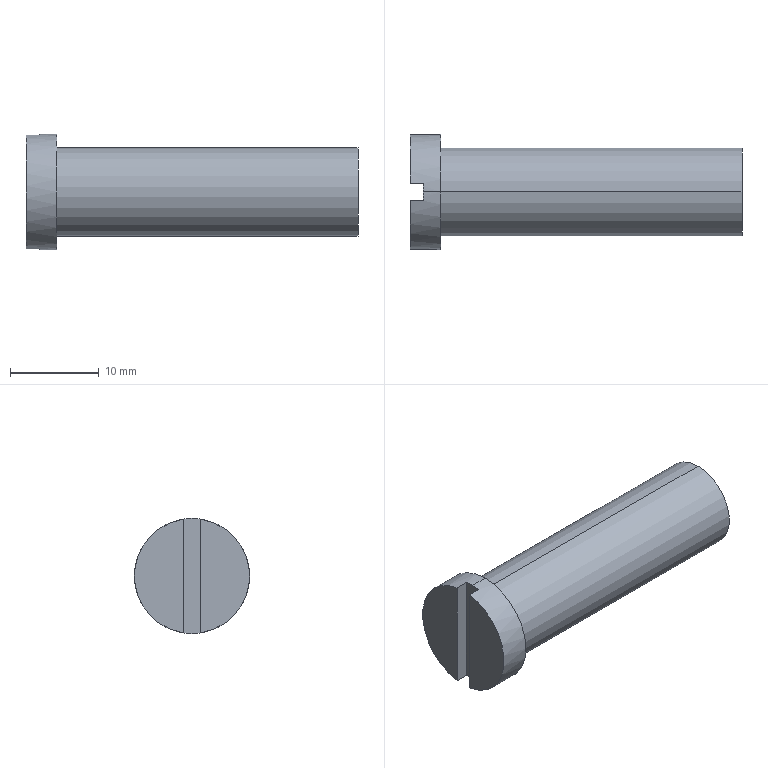Part | SolidWorks | features Chamfer 1, Cut 1, ICE 1, Revolution 1 | 1 solid | 11 faces | box 37.5 x 13 x 13 mm | volume 3096 mm3 | plane 7 | cylinder 4 | commonest cylinder face diameters 10 x2 13 x2
STEP:
#1=CARTESIAN_POINT('',(3.5,0.,6.5));
#2=VERTEX_POINT('',#1);
#3=CARTESIAN_POINT('',(3.5,0.,-6.5));
#4=VERTEX_POINT('',#3);
#5=CARTESIAN_POINT('',(3.5,0.,0.));
#6=DIRECTION('',(-1.,0.,0.));
#7=DIRECTION('',(0.,0.,1.));
#8=AXIS2_PLACEMENT_3D('',#5,#6,#7);
#9=CIRCLE('',#8,6.5);
#10=EDGE_CURVE('',#2,#4,#9,.T.);
#11=ORIENTED_EDGE('',*,*,#10,.T.);
#12=CARTESIAN_POINT('',(1.5,0.,-6.5));
#13=VERTEX_POINT('',#12);
#14=CARTESIAN_POINT('',(-19.421,0.,-6.5));
#15=DIRECTION('',(-1.,0.,0.));
#16=VECTOR('',#15,1000.);
#17=LINE('',#14,#16);
#18=EDGE_CURVE('',#4,#13,#17,.T.);
#19=ORIENTED_EDGE('',*,*,#18,.T.);
#20=CARTESIAN_POINT('',(1.5,1.,-6.423));
#21=VERTEX_POINT('',#20);
#22=CARTESIAN_POINT('',(1.5,0.,0.));
#23=DIRECTION('',(1.,0.,0.));
#24=DIRECTION('',(0.,1.,0.));
#25=AXIS2_PLACEMENT_3D('',#22,#23,#24);
#26=CIRCLE('',#25,6.5);
#27=EDGE_CURVE('',#13,#21,#26,.T.);
#28=ORIENTED_EDGE('',*,*,#27,.T.);
#29=CARTESIAN_POINT('',(0.,1.,-6.423));
#30=VERTEX_POINT('',#29);
#31=CARTESIAN_POINT('',(-19.421,1.,-6.423));
#32=DIRECTION('',(-1.,0.,0.));
#33=VECTOR('',#32,1000.);
#34=LINE('',#31,#33);
#35=EDGE_CURVE('',#21,#30,#34,.T.);
#36=ORIENTED_EDGE('',*,*,#35,.T.);
#37=CARTESIAN_POINT('',(0.,1.,6.423));
#38=VERTEX_POINT('',#37);
#39=CARTESIAN_POINT('',(0.,0.,0.));
#40=DIRECTION('',(-1.,0.,0.));
#41=DIRECTION('',(0.,0.,1.));
#42=AXIS2_PLACEMENT_3D('',#39,#40,#41);
#43=CIRCLE('',#42,6.5);
#44=EDGE_CURVE('',#38,#30,#43,.T.);
#45=ORIENTED_EDGE('',*,*,#44,.F.);
#46=CARTESIAN_POINT('',(1.5,1.,6.423));
#47=VERTEX_POINT('',#46);
#48=CARTESIAN_POINT('',(-19.421,1.,6.423));
#49=DIRECTION('',(1.,0.,0.));
#50=VECTOR('',#49,1000.);
#51=LINE('',#48,#50);
#52=EDGE_CURVE('',#38,#47,#51,.T.);
#53=ORIENTED_EDGE('',*,*,#52,.T.);
#54=CARTESIAN_POINT('',(1.5,0.,6.5));
#55=VERTEX_POINT('',#54);
#56=CARTESIAN_POINT('',(1.5,0.,0.));
#57=DIRECTION('',(1.,0.,0.));
#58=DIRECTION('',(0.,1.,0.));
#59=AXIS2_PLACEMENT_3D('',#56,#57,#58);
#60=CIRCLE('',#59,6.5);
#61=EDGE_CURVE('',#47,#55,#60,.T.);
#62=ORIENTED_EDGE('',*,*,#61,.T.);
#63=CARTESIAN_POINT('',(-19.421,0.,6.5));
#64=DIRECTION('',(-1.,0.,0.));
#65=VECTOR('',#64,1000.);
#66=LINE('',#63,#65);
#67=EDGE_CURVE('',#2,#55,#66,.T.);
#68=ORIENTED_EDGE('',*,*,#67,.F.);
#69=EDGE_LOOP('',(#11,#19,#28,#36,#45,#53,#62,#68));
#70=FACE_OUTER_BOUND('',#69,.T.);
#71=CARTESIAN_POINT('',(-19.421,0.,0.));
#72=DIRECTION('',(-1.,0.,0.));
#73=DIRECTION('',(0.,0.,1.));
#74=AXIS2_PLACEMENT_3D('',#71,#72,#73);
#75=CYLINDRICAL_SURFACE('',#74,6.5);
#76=ADVANCED_FACE('',(#70),#75,.T.);
#77=CARTESIAN_POINT('',(37.5,0.,-5.));
#78=VERTEX_POINT('',#77);
#79=CARTESIAN_POINT('',(37.5,0.,5.));
#80=VERTEX_POINT('',#79);
#81=CARTESIAN_POINT('',(37.5,0.,0.));
#82=DIRECTION('',(1.,0.,0.));
#83=DIRECTION('',(0.,0.,-1.));
#84=AXIS2_PLACEMENT_3D('',#81,#82,#83);
#85=CIRCLE('',#84,5.);
#86=EDGE_CURVE('',#78,#80,#85,.T.);
#87=ORIENTED_EDGE('',*,*,#86,.F.);
#88=CARTESIAN_POINT('',(3.5,0.,-5.));
#89=VERTEX_POINT('',#88);
#90=CARTESIAN_POINT('',(-19.421,0.,-5.));
#91=DIRECTION('',(-1.,0.,0.));
#92=VECTOR('',#91,1000.);
#93=LINE('',#90,#92);
#94=EDGE_CURVE('',#78,#89,#93,.T.);
#95=ORIENTED_EDGE('',*,*,#94,.T.);
#96=CARTESIAN_POINT('',(3.5,0.,5.));
#97=VERTEX_POINT('',#96);
#98=CARTESIAN_POINT('',(3.5,0.,0.));
#99=DIRECTION('',(-1.,0.,0.));
#100=DIRECTION('',(0.,0.,1.));
#101=AXIS2_PLACEMENT_3D('',#98,#99,#100);
#102=CIRCLE('',#101,5.);
#103=EDGE_CURVE('',#97,#89,#102,.T.);
#104=ORIENTED_EDGE('',*,*,#103,.F.);
#105=CARTESIAN_POINT('',(-19.421,0.,5.));
#106=DIRECTION('',(-1.,0.,0.));
#107=VECTOR('',#106,1000.);
#108=LINE('',#105,#107);
#109=EDGE_CURVE('',#80,#97,#108,.T.);
#110=ORIENTED_EDGE('',*,*,#109,.F.);
#111=EDGE_LOOP('',(#87,#95,#104,#110));
#112=FACE_OUTER_BOUND('',#111,.T.);
#113=CARTESIAN_POINT('',(-19.421,0.,0.));
#114=DIRECTION('',(-1.,0.,0.));
#115=DIRECTION('',(0.,0.,1.));
#116=AXIS2_PLACEMENT_3D('',#113,#114,#115);
#117=CYLINDRICAL_SURFACE('',#116,5.);
#118=ADVANCED_FACE('',(#112),#117,.T.);
#119=ORIENTED_EDGE('',*,*,#94,.F.);
#120=CARTESIAN_POINT('',(37.5,0.,0.));
#121=DIRECTION('',(1.,0.,0.));
#122=DIRECTION('',(0.,0.,-1.));
#123=AXIS2_PLACEMENT_3D('',#120,#121,#122);
#124=CIRCLE('',#123,5.);
#125=EDGE_CURVE('',#80,#78,#124,.T.);
#126=ORIENTED_EDGE('',*,*,#125,.F.);
#127=ORIENTED_EDGE('',*,*,#109,.T.);
#128=CARTESIAN_POINT('',(3.5,0.,0.));
#129=DIRECTION('',(-1.,0.,0.));
#130=DIRECTION('',(0.,0.,1.));
#131=AXIS2_PLACEMENT_3D('',#128,#129,#130);
#132=CIRCLE('',#131,5.);
#133=EDGE_CURVE('',#89,#97,#132,.T.);
#134=ORIENTED_EDGE('',*,*,#133,.F.);
#135=EDGE_LOOP('',(#119,#126,#127,#134));
#136=FACE_OUTER_BOUND('',#135,.T.);
#137=CARTESIAN_POINT('',(-19.421,0.,0.));
#138=DIRECTION('',(-1.,0.,0.));
#139=DIRECTION('',(0.,0.,1.));
#140=AXIS2_PLACEMENT_3D('',#137,#138,#139);
#141=CYLINDRICAL_SURFACE('',#140,5.);
#142=ADVANCED_FACE('',(#136),#141,.T.);
#143=CARTESIAN_POINT('',(0.,-1.,-6.423));
#144=VERTEX_POINT('',#143);
#145=CARTESIAN_POINT('',(0.,-1.,6.423));
#146=VERTEX_POINT('',#145);
#147=CARTESIAN_POINT('',(0.,0.,0.));
#148=DIRECTION('',(-1.,0.,0.));
#149=DIRECTION('',(0.,0.,1.));
#150=AXIS2_PLACEMENT_3D('',#147,#148,#149);
#151=CIRCLE('',#150,6.5);
#152=EDGE_CURVE('',#144,#146,#151,.T.);
#153=ORIENTED_EDGE('',*,*,#152,.T.);
#154=CARTESIAN_POINT('',(0.,-1.,-6.5));
#155=DIRECTION('',(0.,0.,1.));
#156=VECTOR('',#155,1000.);
#157=LINE('',#154,#156);
#158=EDGE_CURVE('',#144,#146,#157,.T.);
#159=ORIENTED_EDGE('',*,*,#158,.F.);
#160=EDGE_LOOP('',(#153,#159));
#161=FACE_OUTER_BOUND('',#160,.T.);
#162=CARTESIAN_POINT('',(0.,0.,0.));
#163=DIRECTION('',(1.,0.,0.));
#164=DIRECTION('',(0.,0.,-1.));
#165=AXIS2_PLACEMENT_3D('',#162,#163,#164);
#166=PLANE('',#165);
#167=ADVANCED_FACE('',(#161),#166,.F.);
#168=ORIENTED_EDGE('',*,*,#44,.T.);
#169=CARTESIAN_POINT('',(0.,1.,-6.5));
#170=DIRECTION('',(0.,0.,1.));
#171=VECTOR('',#170,1000.);
#172=LINE('',#169,#171);
#173=EDGE_CURVE('',#30,#38,#172,.T.);
#174=ORIENTED_EDGE('',*,*,#173,.T.);
#175=EDGE_LOOP('',(#168,#174));
#176=FACE_OUTER_BOUND('',#175,.T.);
#177=CARTESIAN_POINT('',(0.,0.,0.));
#178=DIRECTION('',(1.,0.,0.));
#179=DIRECTION('',(0.,0.,-1.));
#180=AXIS2_PLACEMENT_3D('',#177,#178,#179);
#181=PLANE('',#180);
#182=ADVANCED_FACE('',(#176),#181,.F.);
#183=ORIENTED_EDGE('',*,*,#18,.F.);
#184=CARTESIAN_POINT('',(3.5,0.,0.));
#185=DIRECTION('',(-1.,0.,0.));
#186=DIRECTION('',(0.,0.,1.));
#187=AXIS2_PLACEMENT_3D('',#184,#185,#186);
#188=CIRCLE('',#187,6.5);
#189=EDGE_CURVE('',#4,#2,#188,.T.);
#190=ORIENTED_EDGE('',*,*,#189,.T.);
#191=ORIENTED_EDGE('',*,*,#67,.T.);
#192=CARTESIAN_POINT('',(1.5,-1.,6.423));
#193=VERTEX_POINT('',#192);
#194=CARTESIAN_POINT('',(1.5,0.,0.));
#195=DIRECTION('',(1.,0.,0.));
#196=DIRECTION('',(0.,1.,0.));
#197=AXIS2_PLACEMENT_3D('',#194,#195,#196);
#198=CIRCLE('',#197,6.5);
#199=EDGE_CURVE('',#55,#193,#198,.T.);
#200=ORIENTED_EDGE('',*,*,#199,.T.);
#201=CARTESIAN_POINT('',(-19.421,-1.,6.423));
#202=DIRECTION('',(-1.,0.,0.));
#203=VECTOR('',#202,1000.);
#204=LINE('',#201,#203);
#205=EDGE_CURVE('',#193,#146,#204,.T.);
#206=ORIENTED_EDGE('',*,*,#205,.T.);
#207=ORIENTED_EDGE('',*,*,#152,.F.);
#208=CARTESIAN_POINT('',(1.5,-1.,-6.423));
#209=VERTEX_POINT('',#208);
#210=CARTESIAN_POINT('',(-19.421,-1.,-6.423));
#211=DIRECTION('',(1.,0.,0.));
#212=VECTOR('',#211,1000.);
#213=LINE('',#210,#212);
#214=EDGE_CURVE('',#144,#209,#213,.T.);
#215=ORIENTED_EDGE('',*,*,#214,.T.);
#216=CARTESIAN_POINT('',(1.5,0.,0.));
#217=DIRECTION('',(1.,0.,0.));
#218=DIRECTION('',(0.,1.,0.));
#219=AXIS2_PLACEMENT_3D('',#216,#217,#218);
#220=CIRCLE('',#219,6.5);
#221=EDGE_CURVE('',#209,#13,#220,.T.);
#222=ORIENTED_EDGE('',*,*,#221,.T.);
#223=EDGE_LOOP('',(#183,#190,#191,#200,#206,#207,#215,#222));
#224=FACE_OUTER_BOUND('',#223,.T.);
#225=CARTESIAN_POINT('',(-19.421,0.,0.));
#226=DIRECTION('',(-1.,0.,0.));
#227=DIRECTION('',(0.,0.,1.));
#228=AXIS2_PLACEMENT_3D('',#225,#226,#227);
#229=CYLINDRICAL_SURFACE('',#228,6.5);
#230=ADVANCED_FACE('',(#224),#229,.T.);
#231=ORIENTED_EDGE('',*,*,#10,.F.);
#232=ORIENTED_EDGE('',*,*,#189,.F.);
#233=EDGE_LOOP('',(#231,#232));
#234=FACE_OUTER_BOUND('',#233,.T.);
#235=ORIENTED_EDGE('',*,*,#103,.T.);
#236=ORIENTED_EDGE('',*,*,#133,.T.);
#237=EDGE_LOOP('',(#235,#236));
#238=FACE_BOUND('',#237,.T.);
#239=CARTESIAN_POINT('',(3.5,6.5,0.));
#240=DIRECTION('',(-1.,0.,0.));
#241=DIRECTION('',(0.,0.,1.));
#242=AXIS2_PLACEMENT_3D('',#239,#240,#241);
#243=PLANE('',#242);
#244=ADVANCED_FACE('',(#234,#238),#243,.F.);
#245=CARTESIAN_POINT('',(1.5,1.,-6.5));
#246=DIRECTION('',(0.,0.,1.));
#247=VECTOR('',#246,1000.);
#248=LINE('',#245,#247);
#249=EDGE_CURVE('',#21,#47,#248,.T.);
#250=ORIENTED_EDGE('',*,*,#249,.F.);
#251=ORIENTED_EDGE('',*,*,#27,.F.);
#252=ORIENTED_EDGE('',*,*,#221,.F.);
#253=CARTESIAN_POINT('',(1.5,-1.,-6.5));
#254=DIRECTION('',(0.,0.,1.));
#255=VECTOR('',#254,1000.);
#256=LINE('',#253,#255);
#257=EDGE_CURVE('',#209,#193,#256,.T.);
#258=ORIENTED_EDGE('',*,*,#257,.T.);
#259=ORIENTED_EDGE('',*,*,#199,.F.);
#260=ORIENTED_EDGE('',*,*,#61,.F.);
#261=EDGE_LOOP('',(#250,#251,#252,#258,#259,#260));
#262=FACE_OUTER_BOUND('',#261,.T.);
#263=CARTESIAN_POINT('',(1.5,-1.,-6.5));
#264=DIRECTION('',(1.,0.,0.));
#265=DIRECTION('',(0.,1.,0.));
#266=AXIS2_PLACEMENT_3D('',#263,#264,#265);
#267=PLANE('',#266);
#268=ADVANCED_FACE('',(#262),#267,.F.);
#269=ORIENTED_EDGE('',*,*,#257,.F.);
#270=ORIENTED_EDGE('',*,*,#214,.F.);
#271=ORIENTED_EDGE('',*,*,#158,.T.);
#272=ORIENTED_EDGE('',*,*,#205,.F.);
#273=EDGE_LOOP('',(#269,#270,#271,#272));
#274=FACE_OUTER_BOUND('',#273,.T.);
#275=CARTESIAN_POINT('',(1.5,-1.,-6.5));
#276=DIRECTION('',(0.,-1.,0.));
#277=DIRECTION('',(1.,0.,0.));
#278=AXIS2_PLACEMENT_3D('',#275,#276,#277);
#279=PLANE('',#278);
#280=ADVANCED_FACE('',(#274),#279,.F.);
#281=ORIENTED_EDGE('',*,*,#249,.T.);
#282=ORIENTED_EDGE('',*,*,#52,.F.);
#283=ORIENTED_EDGE('',*,*,#173,.F.);
#284=ORIENTED_EDGE('',*,*,#35,.F.);
#285=EDGE_LOOP('',(#281,#282,#283,#284));
#286=FACE_OUTER_BOUND('',#285,.T.);
#287=CARTESIAN_POINT('',(1.5,1.,-6.5));
#288=DIRECTION('',(0.,1.,0.));
#289=DIRECTION('',(-1.,0.,0.));
#290=AXIS2_PLACEMENT_3D('',#287,#288,#289);
#291=PLANE('',#290);
#292=ADVANCED_FACE('',(#286),#291,.F.);
#293=ORIENTED_EDGE('',*,*,#125,.T.);
#294=ORIENTED_EDGE('',*,*,#86,.T.);
#295=EDGE_LOOP('',(#293,#294));
#296=FACE_OUTER_BOUND('',#295,.T.);
#297=CARTESIAN_POINT('',(37.5,0.,0.));
#298=DIRECTION('',(1.,0.,0.));
#299=DIRECTION('',(0.,0.,-1.));
#300=AXIS2_PLACEMENT_3D('',#297,#298,#299);
#301=PLANE('',#300);
#302=ADVANCED_FACE('',(#296),#301,.T.);
#303=CLOSED_SHELL('',(#76,#118,#142,#167,#182,#230,#244,#268,#280,#292,#302));
#304=MANIFOLD_SOLID_BREP('',#303);
#305=CARTESIAN_POINT('',(0.,0.,0.));
#306=DIRECTION('',(0.,0.,1.));
#307=DIRECTION('',(1.,0.,0.));
#308=AXIS2_PLACEMENT_3D('',#305,#306,#307);
#309=(LENGTH_UNIT()NAMED_UNIT(*)SI_UNIT(.MILLI.,.METRE.));
#310=UNCERTAINTY_MEASURE_WITH_UNIT(LENGTH_MEASURE(0.00001),#309,'','');
#311=(NAMED_UNIT(*)PLANE_ANGLE_UNIT()SI_UNIT($,.RADIAN.));
#312=(NAMED_UNIT(*)SI_UNIT($,.STERADIAN.)SOLID_ANGLE_UNIT());
#313=(GEOMETRIC_REPRESENTATION_CONTEXT(3)GLOBAL_UNCERTAINTY_ASSIGNED_CONTEXT((#310))GLOBAL_UNIT_ASSIGNED_CONTEXT((#309,#311,#312))REPRESENTATION_CONTEXT('',''));
#314=ADVANCED_BREP_SHAPE_REPRESENTATION('',(#304,#308),#313);